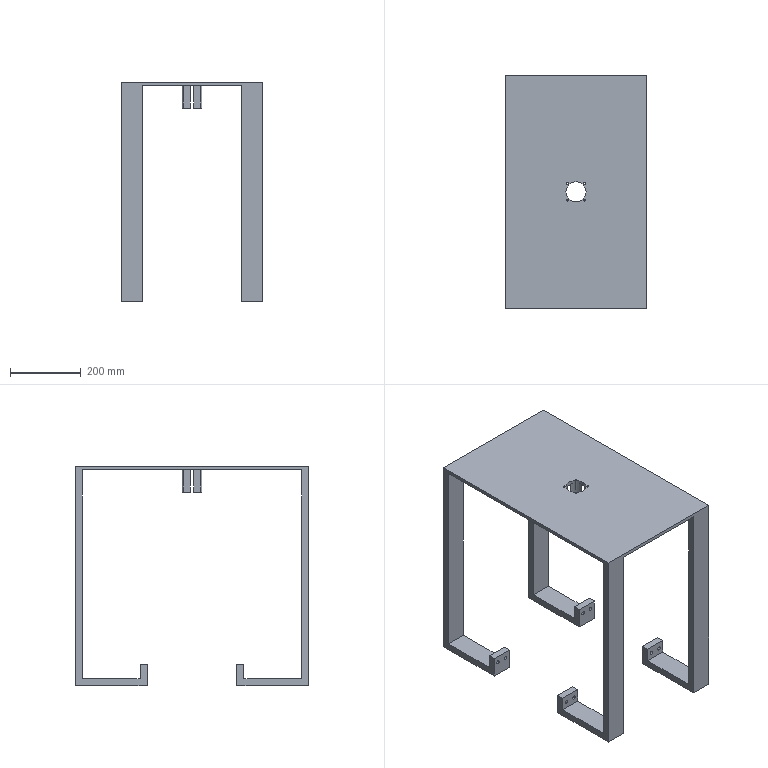Part | SolidWorks | features MirrorPattern 6, ICE 5, Cut 1, Extrusion 1 | 1 solid | 76 faces | box 400 x 660 x 620 mm | volume 6630473 mm3 | plane 46 | cylinder 30 | commonest cylinder face diameters 10 x16 5.2 x8 9 x4 57 x2